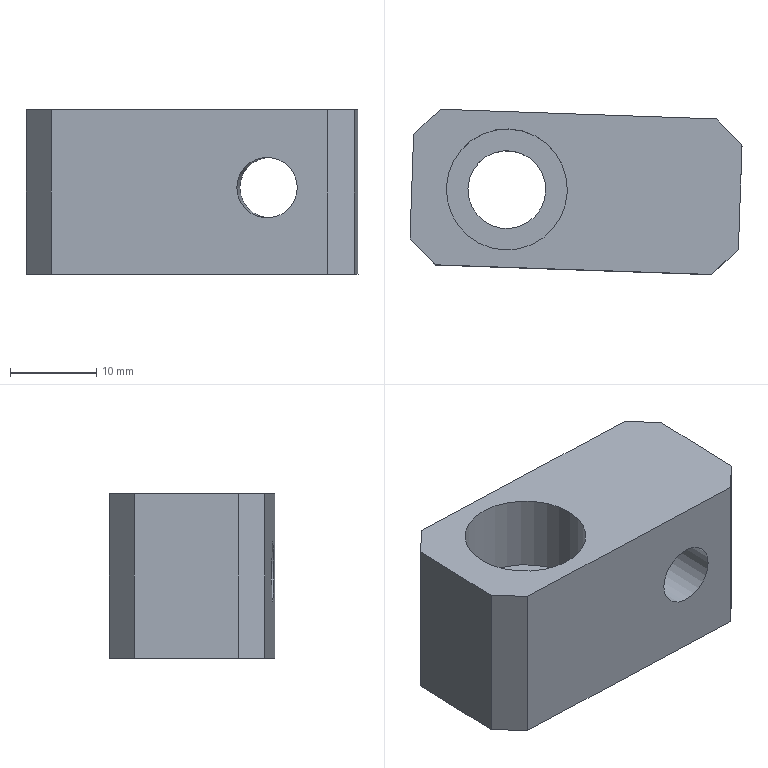Part | NX | features LB-20 2 | 1 solid | 16 faces | box 38.396 x 19.106 x 19 mm | volume 9487 mm3 | plane 12 | cylinder 4 | commonest cylinder face diameters 7 x1 9 x1 11 x1 14 x1
STEP:
#1=CARTESIAN_POINT('',(3808.688,-920.595,793.216));
#2=VERTEX_POINT('',#1);
#3=CARTESIAN_POINT('',(3805.19,-920.473,793.216));
#4=DIRECTION('',(-0.0349,-0.9994,0.));
#5=DIRECTION('',(0.9994,-0.0349,0.000000002));
#6=AXIS2_PLACEMENT_3D('',#3,#4,#5);
#7=CIRCLE('',#6,3.5);
#8=EDGE_CURVE('',#2,#2,#7,.T.);
#9=ORIENTED_EDGE('',*,*,#8,.F.);
#10=EDGE_LOOP('',(#9));
#11=FACE_BOUND('',#10,.T.);
#12=CARTESIAN_POINT('',(3780.205,-919.601,802.216));
#13=VERTEX_POINT('',#12);
#14=CARTESIAN_POINT('',(3812.186,-920.718,802.216));
#15=VERTEX_POINT('',#14);
#16=CARTESIAN_POINT('',(3754.221,-918.694,802.216));
#17=DIRECTION('',(0.9994,-0.0349,0.000000002));
#18=VECTOR('',#17,1000.);
#19=LINE('',#16,#18);
#20=EDGE_CURVE('',#13,#15,#19,.T.);
#21=ORIENTED_EDGE('',*,*,#20,.F.);
#22=CARTESIAN_POINT('',(3780.205,-919.601,783.216));
#23=VERTEX_POINT('',#22);
#24=CARTESIAN_POINT('',(3780.205,-919.601,802.216));
#25=DIRECTION('',(-0.000000002,0.,1.));
#26=VECTOR('',#25,1000.);
#27=LINE('',#24,#26);
#28=EDGE_CURVE('',#23,#13,#27,.T.);
#29=ORIENTED_EDGE('',*,*,#28,.F.);
#30=CARTESIAN_POINT('',(3812.186,-920.718,783.216));
#31=VERTEX_POINT('',#30);
#32=CARTESIAN_POINT('',(3754.221,-918.694,783.216));
#33=DIRECTION('',(0.9994,-0.0349,0.000000002));
#34=VECTOR('',#33,1000.);
#35=LINE('',#32,#34);
#36=EDGE_CURVE('',#23,#31,#35,.T.);
#37=ORIENTED_EDGE('',*,*,#36,.T.);
#38=CARTESIAN_POINT('',(3812.186,-920.718,802.216));
#39=DIRECTION('',(0.000000002,0.,-1.));
#40=VECTOR('',#39,1000.);
#41=LINE('',#38,#40);
#42=EDGE_CURVE('',#15,#31,#41,.T.);
#43=ORIENTED_EDGE('',*,*,#42,.F.);
#44=EDGE_LOOP('',(#21,#29,#37,#43));
#45=FACE_BOUND('',#44,.T.);
#46=CARTESIAN_POINT('',(3754.221,-918.694,802.216));
#47=DIRECTION('',(-0.0349,-0.9994,0.));
#48=DIRECTION('',(0.9994,-0.0349,0.000000002));
#49=AXIS2_PLACEMENT_3D('',#46,#47,#48);
#50=PLANE('',#49);
#51=ADVANCED_FACE('',(#11,#45),#50,.T.);
#52=CARTESIAN_POINT('',(3800.322,-902.292,793.216));
#53=VERTEX_POINT('',#52);
#54=CARTESIAN_POINT('',(3805.818,-902.484,793.216));
#55=DIRECTION('',(0.0349,0.9994,0.));
#56=DIRECTION('',(-0.9994,0.0349,0.));
#57=AXIS2_PLACEMENT_3D('',#54,#55,#56);
#58=CIRCLE('',#57,5.5);
#59=EDGE_CURVE('',#53,#53,#58,.F.);
#60=ORIENTED_EDGE('',*,*,#59,.T.);
#61=EDGE_LOOP('',(#60));
#62=FACE_BOUND('',#61,.T.);
#63=CARTESIAN_POINT('',(3812.814,-902.729,783.216));
#64=VERTEX_POINT('',#63);
#65=CARTESIAN_POINT('',(3780.834,-901.612,783.216));
#66=VERTEX_POINT('',#65);
#67=CARTESIAN_POINT('',(3775.837,-901.437,783.216));
#68=DIRECTION('',(-0.9994,0.0349,-0.000000002));
#69=VECTOR('',#68,1000.);
#70=LINE('',#67,#69);
#71=EDGE_CURVE('',#64,#66,#70,.T.);
#72=ORIENTED_EDGE('',*,*,#71,.T.);
#73=CARTESIAN_POINT('',(3780.834,-901.612,802.216));
#74=VERTEX_POINT('',#73);
#75=CARTESIAN_POINT('',(3780.834,-901.612,799.216));
#76=DIRECTION('',(-0.000000002,0.,1.));
#77=VECTOR('',#76,1000.);
#78=LINE('',#75,#77);
#79=EDGE_CURVE('',#66,#74,#78,.T.);
#80=ORIENTED_EDGE('',*,*,#79,.T.);
#81=CARTESIAN_POINT('',(3812.814,-902.729,802.216));
#82=VERTEX_POINT('',#81);
#83=CARTESIAN_POINT('',(3775.837,-901.437,802.216));
#84=DIRECTION('',(0.9994,-0.0349,0.000000002));
#85=VECTOR('',#84,1000.);
#86=LINE('',#83,#85);
#87=EDGE_CURVE('',#74,#82,#86,.T.);
#88=ORIENTED_EDGE('',*,*,#87,.T.);
#89=CARTESIAN_POINT('',(3812.814,-902.729,799.216));
#90=DIRECTION('',(0.000000002,0.,-1.));
#91=VECTOR('',#90,1000.);
#92=LINE('',#89,#91);
#93=EDGE_CURVE('',#82,#64,#92,.T.);
#94=ORIENTED_EDGE('',*,*,#93,.T.);
#95=EDGE_LOOP('',(#72,#80,#88,#94));
#96=FACE_BOUND('',#95,.T.);
#97=CARTESIAN_POINT('',(3775.837,-901.437,799.216));
#98=DIRECTION('',(0.0349,0.9994,0.));
#99=DIRECTION('',(-0.9994,0.0349,-0.000000002));
#100=AXIS2_PLACEMENT_3D('',#97,#98,#99);
#101=PLANE('',#100);
#102=ADVANCED_FACE('',(#62,#96),#101,.T.);
#103=CARTESIAN_POINT('',(3795.51,-911.13,802.216));
#104=VERTEX_POINT('',#103);
#105=CARTESIAN_POINT('',(3788.515,-910.886,802.216));
#106=DIRECTION('',(-0.000000002,0.,1.));
#107=DIRECTION('',(0.9994,-0.0349,0.000000002));
#108=AXIS2_PLACEMENT_3D('',#105,#106,#107);
#109=CIRCLE('',#108,7.);
#110=EDGE_CURVE('',#104,#104,#109,.T.);
#111=ORIENTED_EDGE('',*,*,#110,.F.);
#112=EDGE_LOOP('',(#111));
#113=FACE_BOUND('',#112,.T.);
#114=ORIENTED_EDGE('',*,*,#87,.F.);
#115=CARTESIAN_POINT('',(3777.731,-904.505,802.216));
#116=VERTEX_POINT('',#115);
#117=CARTESIAN_POINT('',(3767.388,-914.15,802.216));
#118=DIRECTION('',(0.7314,0.682,0.000000001));
#119=VECTOR('',#118,1000.);
#120=LINE('',#117,#119);
#121=EDGE_CURVE('',#74,#116,#120,.F.);
#122=ORIENTED_EDGE('',*,*,#121,.T.);
#123=CARTESIAN_POINT('',(3777.312,-916.498,802.216));
#124=VERTEX_POINT('',#123);
#125=CARTESIAN_POINT('',(3777.556,-909.502,802.216));
#126=DIRECTION('',(0.0349,0.9994,0.));
#127=VECTOR('',#126,1000.);
#128=LINE('',#125,#127);
#129=EDGE_CURVE('',#124,#116,#128,.T.);
#130=ORIENTED_EDGE('',*,*,#129,.F.);
#131=CARTESIAN_POINT('',(3757.54,-895.295,802.216));
#132=DIRECTION('',(-0.682,0.7314,-0.000000001));
#133=VECTOR('',#132,1000.);
#134=LINE('',#131,#133);
#135=EDGE_CURVE('',#13,#124,#134,.T.);
#136=ORIENTED_EDGE('',*,*,#135,.F.);
#137=ORIENTED_EDGE('',*,*,#20,.T.);
#138=CARTESIAN_POINT('',(3815.289,-917.824,802.216));
#139=VERTEX_POINT('',#138);
#140=CARTESIAN_POINT('',(3791.5,-940.007,802.216));
#141=DIRECTION('',(-0.7314,-0.682,-0.000000001));
#142=VECTOR('',#141,1000.);
#143=LINE('',#140,#142);
#144=EDGE_CURVE('',#139,#15,#143,.T.);
#145=ORIENTED_EDGE('',*,*,#144,.F.);
#146=CARTESIAN_POINT('',(3815.708,-905.831,802.216));
#147=VERTEX_POINT('',#146);
#148=CARTESIAN_POINT('',(3815.533,-910.828,802.216));
#149=DIRECTION('',(-0.0349,-0.9994,0.));
#150=VECTOR('',#149,1000.);
#151=LINE('',#148,#150);
#152=EDGE_CURVE('',#147,#139,#151,.T.);
#153=ORIENTED_EDGE('',*,*,#152,.F.);
#154=CARTESIAN_POINT('',(3784.844,-872.734,802.216));
#155=DIRECTION('',(0.682,-0.7314,0.000000001));
#156=VECTOR('',#155,1000.);
#157=LINE('',#154,#156);
#158=EDGE_CURVE('',#147,#82,#157,.F.);
#159=ORIENTED_EDGE('',*,*,#158,.T.);
#160=EDGE_LOOP('',(#114,#122,#130,#136,#137,#145,#153,#159));
#161=FACE_BOUND('',#160,.T.);
#162=CARTESIAN_POINT('',(3754.849,-900.705,802.216));
#163=DIRECTION('',(-0.000000002,0.,1.));
#164=DIRECTION('',(-0.9994,0.0349,-0.000000002));
#165=AXIS2_PLACEMENT_3D('',#162,#163,#164);
#166=PLANE('',#165);
#167=ADVANCED_FACE('',(#113,#161),#166,.T.);
#168=CARTESIAN_POINT('',(3784.017,-910.729,783.216));
#169=VERTEX_POINT('',#168);
#170=CARTESIAN_POINT('',(3788.515,-910.886,783.216));
#171=DIRECTION('',(0.000000002,0.,-1.));
#172=DIRECTION('',(-0.9994,0.0349,-0.000000002));
#173=AXIS2_PLACEMENT_3D('',#170,#171,#172);
#174=CIRCLE('',#173,4.5);
#175=EDGE_CURVE('',#169,#169,#174,.T.);
#176=ORIENTED_EDGE('',*,*,#175,.F.);
#177=EDGE_LOOP('',(#176));
#178=FACE_BOUND('',#177,.T.);
#179=CARTESIAN_POINT('',(3777.731,-904.505,783.216));
#180=VERTEX_POINT('',#179);
#181=CARTESIAN_POINT('',(3777.312,-916.498,783.216));
#182=VERTEX_POINT('',#181);
#183=CARTESIAN_POINT('',(3777.835,-901.507,783.216));
#184=DIRECTION('',(-0.0349,-0.9994,0.));
#185=VECTOR('',#184,1000.);
#186=LINE('',#183,#185);
#187=EDGE_CURVE('',#180,#182,#186,.T.);
#188=ORIENTED_EDGE('',*,*,#187,.F.);
#189=CARTESIAN_POINT('',(3767.388,-914.15,783.216));
#190=DIRECTION('',(-0.7314,-0.682,-0.000000001));
#191=VECTOR('',#190,1000.);
#192=LINE('',#189,#191);
#193=EDGE_CURVE('',#180,#66,#192,.F.);
#194=ORIENTED_EDGE('',*,*,#193,.T.);
#195=ORIENTED_EDGE('',*,*,#71,.F.);
#196=CARTESIAN_POINT('',(3815.708,-905.831,783.216));
#197=VERTEX_POINT('',#196);
#198=CARTESIAN_POINT('',(3784.844,-872.734,783.216));
#199=DIRECTION('',(-0.682,0.7314,-0.000000001));
#200=VECTOR('',#199,1000.);
#201=LINE('',#198,#200);
#202=EDGE_CURVE('',#64,#197,#201,.F.);
#203=ORIENTED_EDGE('',*,*,#202,.T.);
#204=CARTESIAN_POINT('',(3815.289,-917.824,783.216));
#205=VERTEX_POINT('',#204);
#206=CARTESIAN_POINT('',(3815.812,-902.833,783.216));
#207=DIRECTION('',(0.0349,0.9994,0.));
#208=VECTOR('',#207,1000.);
#209=LINE('',#206,#208);
#210=EDGE_CURVE('',#205,#197,#209,.T.);
#211=ORIENTED_EDGE('',*,*,#210,.F.);
#212=CARTESIAN_POINT('',(3801.843,-930.363,783.216));
#213=DIRECTION('',(0.7314,0.682,0.000000001));
#214=VECTOR('',#213,1000.);
#215=LINE('',#212,#214);
#216=EDGE_CURVE('',#31,#205,#215,.T.);
#217=ORIENTED_EDGE('',*,*,#216,.F.);
#218=ORIENTED_EDGE('',*,*,#36,.F.);
#219=CARTESIAN_POINT('',(3759.951,-897.881,783.216));
#220=DIRECTION('',(0.682,-0.7314,0.000000001));
#221=VECTOR('',#220,1000.);
#222=LINE('',#219,#221);
#223=EDGE_CURVE('',#182,#23,#222,.T.);
#224=ORIENTED_EDGE('',*,*,#223,.F.);
#225=EDGE_LOOP('',(#188,#194,#195,#203,#211,#217,#218,#224));
#226=FACE_BOUND('',#225,.T.);
#227=CARTESIAN_POINT('',(3754.849,-900.705,783.216));
#228=DIRECTION('',(0.000000002,0.,-1.));
#229=DIRECTION('',(0.9994,-0.0349,0.000000002));
#230=AXIS2_PLACEMENT_3D('',#227,#228,#229);
#231=PLANE('',#230);
#232=ADVANCED_FACE('',(#178,#226),#231,.T.);
#233=CARTESIAN_POINT('',(3784.017,-910.729,793.216));
#234=VERTEX_POINT('',#233);
#235=CARTESIAN_POINT('',(3788.515,-910.886,793.216));
#236=DIRECTION('',(0.000000002,0.,-1.));
#237=DIRECTION('',(-0.9994,0.0349,-0.000000002));
#238=AXIS2_PLACEMENT_3D('',#235,#236,#237);
#239=CIRCLE('',#238,4.5);
#240=EDGE_CURVE('',#234,#234,#239,.T.);
#241=ORIENTED_EDGE('',*,*,#240,.F.);
#242=EDGE_LOOP('',(#241));
#243=FACE_BOUND('',#242,.T.);
#244=ORIENTED_EDGE('',*,*,#175,.T.);
#245=EDGE_LOOP('',(#244));
#246=FACE_BOUND('',#245,.T.);
#247=CARTESIAN_POINT('',(3788.515,-910.886,791.216));
#248=DIRECTION('',(-0.000000002,0.,1.));
#249=DIRECTION('',(-0.9994,0.0349,-0.000000002));
#250=AXIS2_PLACEMENT_3D('',#247,#248,#249);
#251=CYLINDRICAL_SURFACE('',#250,4.5);
#252=ADVANCED_FACE('',(#243,#246),#251,.F.);
#253=ORIENTED_EDGE('',*,*,#240,.T.);
#254=EDGE_LOOP('',(#253));
#255=FACE_BOUND('',#254,.T.);
#256=CARTESIAN_POINT('',(3795.51,-911.13,793.216));
#257=VERTEX_POINT('',#256);
#258=CARTESIAN_POINT('',(3788.515,-910.886,793.216));
#259=DIRECTION('',(0.000000002,0.,-1.));
#260=DIRECTION('',(0.9994,-0.0349,0.000000002));
#261=AXIS2_PLACEMENT_3D('',#258,#259,#260);
#262=CIRCLE('',#261,7.);
#263=EDGE_CURVE('',#257,#257,#262,.T.);
#264=ORIENTED_EDGE('',*,*,#263,.F.);
#265=EDGE_LOOP('',(#264));
#266=FACE_BOUND('',#265,.T.);
#267=CARTESIAN_POINT('',(3788.515,-910.886,793.216));
#268=DIRECTION('',(0.000000002,0.,-1.));
#269=DIRECTION('',(0.9994,-0.0349,0.000000002));
#270=AXIS2_PLACEMENT_3D('',#267,#268,#269);
#271=PLANE('',#270);
#272=ADVANCED_FACE('',(#255,#266),#271,.F.);
#273=ORIENTED_EDGE('',*,*,#110,.T.);
#274=EDGE_LOOP('',(#273));
#275=FACE_BOUND('',#274,.T.);
#276=ORIENTED_EDGE('',*,*,#263,.T.);
#277=EDGE_LOOP('',(#276));
#278=FACE_BOUND('',#277,.T.);
#279=CARTESIAN_POINT('',(3788.515,-910.886,798.216));
#280=DIRECTION('',(-0.000000002,0.,1.));
#281=DIRECTION('',(-0.9994,0.0349,-0.000000002));
#282=AXIS2_PLACEMENT_3D('',#279,#280,#281);
#283=CYLINDRICAL_SURFACE('',#282,7.);
#284=ADVANCED_FACE('',(#275,#278),#283,.F.);
#285=ORIENTED_EDGE('',*,*,#210,.T.);
#286=CARTESIAN_POINT('',(3815.708,-905.831,799.216));
#287=DIRECTION('',(-0.000000002,0.,1.));
#288=VECTOR('',#287,1000.);
#289=LINE('',#286,#288);
#290=EDGE_CURVE('',#197,#147,#289,.T.);
#291=ORIENTED_EDGE('',*,*,#290,.T.);
#292=ORIENTED_EDGE('',*,*,#152,.T.);
#293=CARTESIAN_POINT('',(3815.289,-917.824,799.216));
#294=DIRECTION('',(-0.000000002,0.,1.));
#295=VECTOR('',#294,1000.);
#296=LINE('',#293,#295);
#297=EDGE_CURVE('',#205,#139,#296,.T.);
#298=ORIENTED_EDGE('',*,*,#297,.F.);
#299=EDGE_LOOP('',(#285,#291,#292,#298));
#300=FACE_BOUND('',#299,.T.);
#301=CARTESIAN_POINT('',(3815.533,-910.828,799.216));
#302=DIRECTION('',(0.9994,-0.0349,0.000000002));
#303=DIRECTION('',(0.000000002,0.,-1.));
#304=AXIS2_PLACEMENT_3D('',#301,#302,#303);
#305=PLANE('',#304);
#306=ADVANCED_FACE('',(#300),#305,.T.);
#307=ORIENTED_EDGE('',*,*,#129,.T.);
#308=CARTESIAN_POINT('',(3777.731,-904.505,799.216));
#309=DIRECTION('',(0.000000002,0.,-1.));
#310=VECTOR('',#309,1000.);
#311=LINE('',#308,#310);
#312=EDGE_CURVE('',#116,#180,#311,.T.);
#313=ORIENTED_EDGE('',*,*,#312,.T.);
#314=ORIENTED_EDGE('',*,*,#187,.T.);
#315=CARTESIAN_POINT('',(3777.312,-916.498,799.216));
#316=DIRECTION('',(0.000000002,0.,-1.));
#317=VECTOR('',#316,1000.);
#318=LINE('',#315,#317);
#319=EDGE_CURVE('',#124,#182,#318,.T.);
#320=ORIENTED_EDGE('',*,*,#319,.F.);
#321=EDGE_LOOP('',(#307,#313,#314,#320));
#322=FACE_BOUND('',#321,.T.);
#323=CARTESIAN_POINT('',(3777.556,-909.502,799.216));
#324=DIRECTION('',(-0.9994,0.0349,-0.000000002));
#325=DIRECTION('',(-0.000000002,0.,1.));
#326=AXIS2_PLACEMENT_3D('',#323,#324,#325);
#327=PLANE('',#326);
#328=ADVANCED_FACE('',(#322),#327,.T.);
#329=ORIENTED_EDGE('',*,*,#144,.T.);
#330=ORIENTED_EDGE('',*,*,#42,.T.);
#331=ORIENTED_EDGE('',*,*,#216,.T.);
#332=ORIENTED_EDGE('',*,*,#297,.T.);
#333=EDGE_LOOP('',(#329,#330,#331,#332));
#334=FACE_BOUND('',#333,.T.);
#335=CARTESIAN_POINT('',(3812.186,-920.718,802.216));
#336=DIRECTION('',(-0.682,0.7314,-0.000000001));
#337=DIRECTION('',(0.7314,0.682,0.000000001));
#338=AXIS2_PLACEMENT_3D('',#335,#336,#337);
#339=PLANE('',#338);
#340=ADVANCED_FACE('',(#334),#339,.F.);
#341=ORIENTED_EDGE('',*,*,#223,.T.);
#342=ORIENTED_EDGE('',*,*,#28,.T.);
#343=ORIENTED_EDGE('',*,*,#135,.T.);
#344=ORIENTED_EDGE('',*,*,#319,.T.);
#345=EDGE_LOOP('',(#341,#342,#343,#344));
#346=FACE_BOUND('',#345,.T.);
#347=CARTESIAN_POINT('',(3780.205,-919.601,802.216));
#348=DIRECTION('',(0.7314,0.682,0.000000001));
#349=DIRECTION('',(0.682,-0.7314,0.000000001));
#350=AXIS2_PLACEMENT_3D('',#347,#348,#349);
#351=PLANE('',#350);
#352=ADVANCED_FACE('',(#346),#351,.F.);
#353=ORIENTED_EDGE('',*,*,#8,.T.);
#354=EDGE_LOOP('',(#353));
#355=FACE_BOUND('',#354,.T.);
#356=CARTESIAN_POINT('',(3809.037,-910.602,793.216));
#357=VERTEX_POINT('',#356);
#358=CARTESIAN_POINT('',(3805.539,-910.479,793.216));
#359=DIRECTION('',(-0.0349,-0.9994,0.));
#360=DIRECTION('',(0.9994,-0.0349,0.000000002));
#361=AXIS2_PLACEMENT_3D('',#358,#359,#360);
#362=CIRCLE('',#361,3.5);
#363=EDGE_CURVE('',#357,#357,#362,.T.);
#364=ORIENTED_EDGE('',*,*,#363,.F.);
#365=EDGE_LOOP('',(#364));
#366=FACE_BOUND('',#365,.T.);
#367=CARTESIAN_POINT('',(3805.19,-920.473,793.216));
#368=DIRECTION('',(-0.0349,-0.9994,0.));
#369=DIRECTION('',(-0.9994,0.0349,-0.000000002));
#370=AXIS2_PLACEMENT_3D('',#367,#368,#369);
#371=CYLINDRICAL_SURFACE('',#370,3.5);
#372=ADVANCED_FACE('',(#355,#366),#371,.F.);
#373=ORIENTED_EDGE('',*,*,#363,.T.);
#374=EDGE_LOOP('',(#373));
#375=FACE_BOUND('',#374,.T.);
#376=CARTESIAN_POINT('',(3811.036,-910.671,793.216));
#377=VERTEX_POINT('',#376);
#378=CARTESIAN_POINT('',(3805.539,-910.479,793.216));
#379=DIRECTION('',(-0.0349,-0.9994,0.));
#380=DIRECTION('',(0.9994,-0.0349,0.000000002));
#381=AXIS2_PLACEMENT_3D('',#378,#379,#380);
#382=CIRCLE('',#381,5.5);
#383=EDGE_CURVE('',#377,#377,#382,.T.);
#384=ORIENTED_EDGE('',*,*,#383,.F.);
#385=EDGE_LOOP('',(#384));
#386=FACE_BOUND('',#385,.T.);
#387=CARTESIAN_POINT('',(3805.539,-910.479,793.216));
#388=DIRECTION('',(-0.0349,-0.9994,0.));
#389=DIRECTION('',(-0.9994,0.0349,-0.000000002));
#390=AXIS2_PLACEMENT_3D('',#387,#388,#389);
#391=PLANE('',#390);
#392=ADVANCED_FACE('',(#375,#386),#391,.F.);
#393=ORIENTED_EDGE('',*,*,#383,.T.);
#394=EDGE_LOOP('',(#393));
#395=FACE_BOUND('',#394,.T.);
#396=ORIENTED_EDGE('',*,*,#59,.F.);
#397=EDGE_LOOP('',(#396));
#398=FACE_BOUND('',#397,.T.);
#399=CARTESIAN_POINT('',(3805.888,-900.485,793.216));
#400=DIRECTION('',(-0.0349,-0.9994,0.));
#401=DIRECTION('',(-0.9994,0.0349,-0.000000002));
#402=AXIS2_PLACEMENT_3D('',#399,#400,#401);
#403=CYLINDRICAL_SURFACE('',#402,5.5);
#404=ADVANCED_FACE('',(#395,#398),#403,.F.);
#405=ORIENTED_EDGE('',*,*,#193,.F.);
#406=ORIENTED_EDGE('',*,*,#312,.F.);
#407=ORIENTED_EDGE('',*,*,#121,.F.);
#408=ORIENTED_EDGE('',*,*,#79,.F.);
#409=EDGE_LOOP('',(#405,#406,#407,#408));
#410=FACE_BOUND('',#409,.T.);
#411=CARTESIAN_POINT('',(3780.834,-901.612,799.216));
#412=DIRECTION('',(0.682,-0.7314,0.000000001));
#413=DIRECTION('',(-0.000000002,0.,1.));
#414=AXIS2_PLACEMENT_3D('',#411,#412,#413);
#415=PLANE('',#414);
#416=ADVANCED_FACE('',(#410),#415,.F.);
#417=ORIENTED_EDGE('',*,*,#158,.F.);
#418=ORIENTED_EDGE('',*,*,#290,.F.);
#419=ORIENTED_EDGE('',*,*,#202,.F.);
#420=ORIENTED_EDGE('',*,*,#93,.F.);
#421=EDGE_LOOP('',(#417,#418,#419,#420));
#422=FACE_BOUND('',#421,.T.);
#423=CARTESIAN_POINT('',(3812.814,-902.729,799.216));
#424=DIRECTION('',(-0.7314,-0.682,-0.000000001));
#425=DIRECTION('',(0.000000002,0.,-1.));
#426=AXIS2_PLACEMENT_3D('',#423,#424,#425);
#427=PLANE('',#426);
#428=ADVANCED_FACE('',(#422),#427,.F.);
#429=CLOSED_SHELL('',(#51,#102,#167,#232,#252,#272,#284,#306,#328,#340,#352,#372,#392,#404,#416,#428));
#430=MANIFOLD_SOLID_BREP('',#429);
#431=(LENGTH_UNIT()NAMED_UNIT(*)SI_UNIT(.MILLI.,.METRE.));
#432=UNCERTAINTY_MEASURE_WITH_UNIT(LENGTH_MEASURE(0.00001),#431,'','');
#433=(NAMED_UNIT(*)PLANE_ANGLE_UNIT()SI_UNIT($,.RADIAN.));
#434=(NAMED_UNIT(*)SI_UNIT($,.STERADIAN.)SOLID_ANGLE_UNIT());
#435=(GEOMETRIC_REPRESENTATION_CONTEXT(3)GLOBAL_UNCERTAINTY_ASSIGNED_CONTEXT((#432))GLOBAL_UNIT_ASSIGNED_CONTEXT((#431,#433,#434))REPRESENTATION_CONTEXT('',''));
#436=ADVANCED_BREP_SHAPE_REPRESENTATION('',(#430),#435);